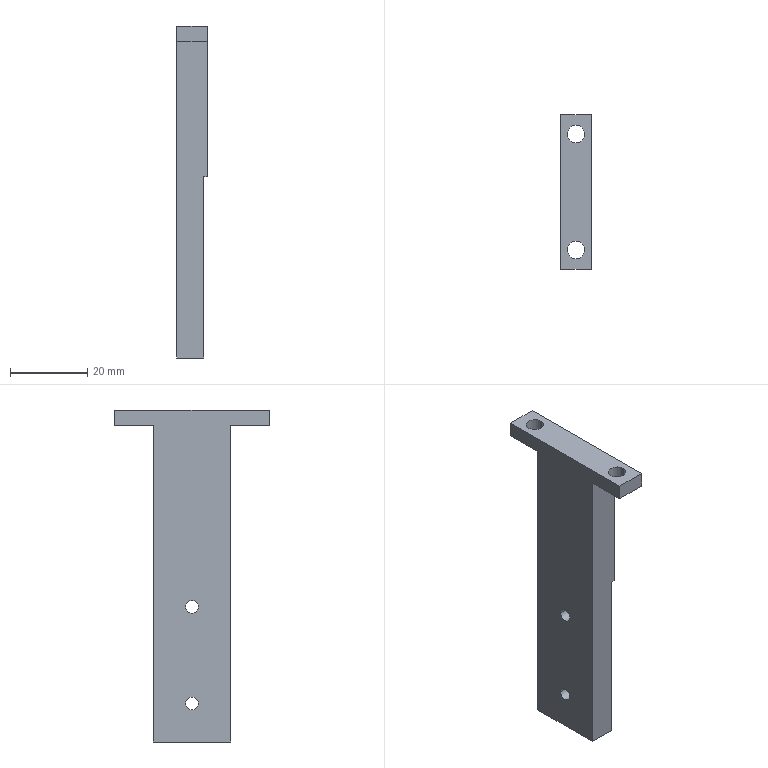Part | NX | 1 solid | 24 faces | box 8 x 40 x 86 mm | volume 13210 mm3 | plane 12 | cylinder 8 | cone 4 | commonest cylinder face diameters 3.3 x4 4.5 x4
STEP:
#1=CARTESIAN_POINT('',(7.,0.,0.));
#2=VERTEX_POINT('',#1);
#3=CARTESIAN_POINT('',(7.,-20.,0.));
#4=VERTEX_POINT('',#3);
#5=CARTESIAN_POINT('',(7.,0.,0.));
#6=DIRECTION('',(0.,-1.,0.));
#7=VECTOR('',#6,1000.);
#8=LINE('',#5,#7);
#9=EDGE_CURVE('',#2,#4,#8,.T.);
#10=ORIENTED_EDGE('',*,*,#9,.T.);
#11=CARTESIAN_POINT('',(0.,-20.,0.));
#12=VERTEX_POINT('',#11);
#13=CARTESIAN_POINT('',(7.,-20.,0.));
#14=DIRECTION('',(-1.,0.,0.));
#15=VECTOR('',#14,1000.);
#16=LINE('',#13,#15);
#17=EDGE_CURVE('',#4,#12,#16,.T.);
#18=ORIENTED_EDGE('',*,*,#17,.T.);
#19=CARTESIAN_POINT('',(0.,0.,0.));
#20=VERTEX_POINT('',#19);
#21=CARTESIAN_POINT('',(0.,0.,0.));
#22=DIRECTION('',(0.,-1.,0.));
#23=VECTOR('',#22,1000.);
#24=LINE('',#21,#23);
#25=EDGE_CURVE('',#20,#12,#24,.T.);
#26=ORIENTED_EDGE('',*,*,#25,.F.);
#27=CARTESIAN_POINT('',(0.,0.,0.));
#28=DIRECTION('',(1.,0.,0.));
#29=VECTOR('',#28,1000.);
#30=LINE('',#27,#29);
#31=EDGE_CURVE('',#20,#2,#30,.T.);
#32=ORIENTED_EDGE('',*,*,#31,.T.);
#33=EDGE_LOOP('',(#10,#18,#26,#32));
#34=FACE_BOUND('',#33,.T.);
#35=CARTESIAN_POINT('',(0.,0.,0.));
#36=DIRECTION('',(0.,0.,1.));
#37=DIRECTION('',(1.,0.,0.));
#38=AXIS2_PLACEMENT_3D('',#35,#36,#37);
#39=PLANE('',#38);
#40=ADVANCED_FACE('',(#34),#39,.F.);
#41=ORIENTED_EDGE('',*,*,#9,.F.);
#42=CARTESIAN_POINT('',(7.,0.,47.));
#43=VERTEX_POINT('',#42);
#44=CARTESIAN_POINT('',(7.,0.,0.));
#45=DIRECTION('',(0.,0.,1.));
#46=VECTOR('',#45,1000.);
#47=LINE('',#44,#46);
#48=EDGE_CURVE('',#2,#43,#47,.T.);
#49=ORIENTED_EDGE('',*,*,#48,.T.);
#50=CARTESIAN_POINT('',(7.,-20.,47.));
#51=VERTEX_POINT('',#50);
#52=CARTESIAN_POINT('',(7.,0.,47.));
#53=DIRECTION('',(0.,-1.,0.));
#54=VECTOR('',#53,1000.);
#55=LINE('',#52,#54);
#56=EDGE_CURVE('',#43,#51,#55,.T.);
#57=ORIENTED_EDGE('',*,*,#56,.T.);
#58=CARTESIAN_POINT('',(7.,-20.,0.));
#59=DIRECTION('',(0.,0.,-1.));
#60=VECTOR('',#59,1000.);
#61=LINE('',#58,#60);
#62=EDGE_CURVE('',#51,#4,#61,.T.);
#63=ORIENTED_EDGE('',*,*,#62,.T.);
#64=EDGE_LOOP('',(#41,#49,#57,#63));
#65=FACE_BOUND('',#64,.T.);
#66=CARTESIAN_POINT('',(7.,-7.685,35.));
#67=VERTEX_POINT('',#66);
#68=CARTESIAN_POINT('',(7.,-12.315,35.));
#69=VERTEX_POINT('',#68);
#70=CARTESIAN_POINT('',(7.,-10.,35.));
#71=DIRECTION('',(1.,0.,0.));
#72=DIRECTION('',(0.,-1.,0.));
#73=AXIS2_PLACEMENT_3D('',#70,#71,#72);
#74=CIRCLE('',#73,2.315);
#75=EDGE_CURVE('',#67,#69,#74,.T.);
#76=ORIENTED_EDGE('',*,*,#75,.F.);
#77=CARTESIAN_POINT('',(7.,-10.,35.));
#78=DIRECTION('',(1.,0.,0.));
#79=DIRECTION('',(0.,-1.,0.));
#80=AXIS2_PLACEMENT_3D('',#77,#78,#79);
#81=CIRCLE('',#80,2.315);
#82=EDGE_CURVE('',#69,#67,#81,.T.);
#83=ORIENTED_EDGE('',*,*,#82,.F.);
#84=EDGE_LOOP('',(#76,#83));
#85=FACE_BOUND('',#84,.T.);
#86=CARTESIAN_POINT('',(7.,-7.685,10.));
#87=VERTEX_POINT('',#86);
#88=CARTESIAN_POINT('',(7.,-12.315,10.));
#89=VERTEX_POINT('',#88);
#90=CARTESIAN_POINT('',(7.,-10.,10.));
#91=DIRECTION('',(1.,0.,0.));
#92=DIRECTION('',(0.,-1.,0.));
#93=AXIS2_PLACEMENT_3D('',#90,#91,#92);
#94=CIRCLE('',#93,2.315);
#95=EDGE_CURVE('',#87,#89,#94,.T.);
#96=ORIENTED_EDGE('',*,*,#95,.F.);
#97=CARTESIAN_POINT('',(7.,-10.,10.));
#98=DIRECTION('',(1.,0.,0.));
#99=DIRECTION('',(0.,-1.,0.));
#100=AXIS2_PLACEMENT_3D('',#97,#98,#99);
#101=CIRCLE('',#100,2.315);
#102=EDGE_CURVE('',#89,#87,#101,.T.);
#103=ORIENTED_EDGE('',*,*,#102,.F.);
#104=EDGE_LOOP('',(#96,#103));
#105=FACE_BOUND('',#104,.T.);
#106=CARTESIAN_POINT('',(7.,0.,0.));
#107=DIRECTION('',(-1.,0.,0.));
#108=DIRECTION('',(0.,0.,1.));
#109=AXIS2_PLACEMENT_3D('',#106,#107,#108);
#110=PLANE('',#109);
#111=ADVANCED_FACE('',(#65,#85,#105),#110,.F.);
#112=CARTESIAN_POINT('',(8.,-20.,82.));
#113=VERTEX_POINT('',#112);
#114=CARTESIAN_POINT('',(0.,-20.,82.));
#115=VERTEX_POINT('',#114);
#116=CARTESIAN_POINT('',(8.,-20.,82.));
#117=DIRECTION('',(-1.,0.,0.));
#118=VECTOR('',#117,1000.);
#119=LINE('',#116,#118);
#120=EDGE_CURVE('',#113,#115,#119,.T.);
#121=ORIENTED_EDGE('',*,*,#120,.T.);
#122=CARTESIAN_POINT('',(0.,-20.,0.));
#123=DIRECTION('',(0.,0.,-1.));
#124=VECTOR('',#123,1000.);
#125=LINE('',#122,#124);
#126=EDGE_CURVE('',#115,#12,#125,.T.);
#127=ORIENTED_EDGE('',*,*,#126,.T.);
#128=ORIENTED_EDGE('',*,*,#17,.F.);
#129=ORIENTED_EDGE('',*,*,#62,.F.);
#130=CARTESIAN_POINT('',(8.,-20.,47.));
#131=VERTEX_POINT('',#130);
#132=CARTESIAN_POINT('',(7.,-20.,47.));
#133=DIRECTION('',(1.,0.,0.));
#134=VECTOR('',#133,1000.);
#135=LINE('',#132,#134);
#136=EDGE_CURVE('',#51,#131,#135,.T.);
#137=ORIENTED_EDGE('',*,*,#136,.T.);
#138=CARTESIAN_POINT('',(8.,-20.,82.));
#139=DIRECTION('',(0.,0.,-1.));
#140=VECTOR('',#139,1000.);
#141=LINE('',#138,#140);
#142=EDGE_CURVE('',#113,#131,#141,.T.);
#143=ORIENTED_EDGE('',*,*,#142,.F.);
#144=EDGE_LOOP('',(#121,#127,#128,#129,#137,#143));
#145=FACE_BOUND('',#144,.T.);
#146=CARTESIAN_POINT('',(0.,-20.,0.));
#147=DIRECTION('',(0.,-1.,0.));
#148=DIRECTION('',(0.,0.,-1.));
#149=AXIS2_PLACEMENT_3D('',#146,#147,#148);
#150=PLANE('',#149);
#151=ADVANCED_FACE('',(#145),#150,.T.);
#152=CARTESIAN_POINT('',(0.,0.,82.));
#153=VERTEX_POINT('',#152);
#154=CARTESIAN_POINT('',(8.,0.,82.));
#155=VERTEX_POINT('',#154);
#156=CARTESIAN_POINT('',(0.,0.,82.));
#157=DIRECTION('',(1.,0.,0.));
#158=VECTOR('',#157,1000.);
#159=LINE('',#156,#158);
#160=EDGE_CURVE('',#153,#155,#159,.T.);
#161=ORIENTED_EDGE('',*,*,#160,.F.);
#162=CARTESIAN_POINT('',(0.,10.,82.));
#163=VERTEX_POINT('',#162);
#164=CARTESIAN_POINT('',(0.,0.,82.));
#165=DIRECTION('',(0.,1.,0.));
#166=VECTOR('',#165,1000.);
#167=LINE('',#164,#166);
#168=EDGE_CURVE('',#153,#163,#167,.T.);
#169=ORIENTED_EDGE('',*,*,#168,.T.);
#170=CARTESIAN_POINT('',(8.,10.,82.));
#171=VERTEX_POINT('',#170);
#172=CARTESIAN_POINT('',(0.,10.,82.));
#173=DIRECTION('',(1.,0.,0.));
#174=VECTOR('',#173,1000.);
#175=LINE('',#172,#174);
#176=EDGE_CURVE('',#163,#171,#175,.T.);
#177=ORIENTED_EDGE('',*,*,#176,.T.);
#178=CARTESIAN_POINT('',(8.,10.,82.));
#179=DIRECTION('',(0.,-1.,0.));
#180=VECTOR('',#179,1000.);
#181=LINE('',#178,#180);
#182=EDGE_CURVE('',#171,#155,#181,.T.);
#183=ORIENTED_EDGE('',*,*,#182,.T.);
#184=EDGE_LOOP('',(#161,#169,#177,#183));
#185=FACE_BOUND('',#184,.T.);
#186=CARTESIAN_POINT('',(1.75,5.,82.));
#187=VERTEX_POINT('',#186);
#188=CARTESIAN_POINT('',(6.25,5.,82.));
#189=VERTEX_POINT('',#188);
#190=CARTESIAN_POINT('',(4.,5.,82.));
#191=DIRECTION('',(0.,0.,-1.));
#192=DIRECTION('',(1.,0.,0.));
#193=AXIS2_PLACEMENT_3D('',#190,#191,#192);
#194=CIRCLE('',#193,2.25);
#195=EDGE_CURVE('',#187,#189,#194,.T.);
#196=ORIENTED_EDGE('',*,*,#195,.F.);
#197=CARTESIAN_POINT('',(4.,5.,82.));
#198=DIRECTION('',(0.,0.,-1.));
#199=DIRECTION('',(1.,0.,0.));
#200=AXIS2_PLACEMENT_3D('',#197,#198,#199);
#201=CIRCLE('',#200,2.25);
#202=EDGE_CURVE('',#189,#187,#201,.T.);
#203=ORIENTED_EDGE('',*,*,#202,.F.);
#204=EDGE_LOOP('',(#196,#203));
#205=FACE_BOUND('',#204,.T.);
#206=CARTESIAN_POINT('',(8.,0.,82.));
#207=DIRECTION('',(0.,0.,-1.));
#208=DIRECTION('',(0.,-1.,0.));
#209=AXIS2_PLACEMENT_3D('',#206,#207,#208);
#210=PLANE('',#209);
#211=ADVANCED_FACE('',(#185,#205),#210,.T.);
#212=CARTESIAN_POINT('',(0.,10.,86.));
#213=VERTEX_POINT('',#212);
#214=CARTESIAN_POINT('',(0.,-30.,86.));
#215=VERTEX_POINT('',#214);
#216=CARTESIAN_POINT('',(0.,0.,86.));
#217=DIRECTION('',(0.,-1.,0.));
#218=VECTOR('',#217,1000.);
#219=LINE('',#216,#218);
#220=EDGE_CURVE('',#213,#215,#219,.T.);
#221=ORIENTED_EDGE('',*,*,#220,.F.);
#222=CARTESIAN_POINT('',(0.,10.,0.));
#223=DIRECTION('',(0.,0.,1.));
#224=VECTOR('',#223,1000.);
#225=LINE('',#222,#224);
#226=EDGE_CURVE('',#163,#213,#225,.T.);
#227=ORIENTED_EDGE('',*,*,#226,.F.);
#228=ORIENTED_EDGE('',*,*,#168,.F.);
#229=CARTESIAN_POINT('',(0.,0.,0.));
#230=DIRECTION('',(0.,0.,1.));
#231=VECTOR('',#230,1000.);
#232=LINE('',#229,#231);
#233=EDGE_CURVE('',#20,#153,#232,.T.);
#234=ORIENTED_EDGE('',*,*,#233,.F.);
#235=ORIENTED_EDGE('',*,*,#25,.T.);
#236=ORIENTED_EDGE('',*,*,#126,.F.);
#237=CARTESIAN_POINT('',(0.,-30.,82.));
#238=VERTEX_POINT('',#237);
#239=CARTESIAN_POINT('',(0.,0.,82.));
#240=DIRECTION('',(0.,1.,0.));
#241=VECTOR('',#240,1000.);
#242=LINE('',#239,#241);
#243=EDGE_CURVE('',#238,#115,#242,.T.);
#244=ORIENTED_EDGE('',*,*,#243,.F.);
#245=CARTESIAN_POINT('',(0.,-30.,0.));
#246=DIRECTION('',(0.,0.,-1.));
#247=VECTOR('',#246,1000.);
#248=LINE('',#245,#247);
#249=EDGE_CURVE('',#215,#238,#248,.T.);
#250=ORIENTED_EDGE('',*,*,#249,.F.);
#251=EDGE_LOOP('',(#221,#227,#228,#234,#235,#236,#244,#250));
#252=FACE_BOUND('',#251,.T.);
#253=CARTESIAN_POINT('',(0.,-11.65,35.));
#254=VERTEX_POINT('',#253);
#255=CARTESIAN_POINT('',(0.,-8.35,35.));
#256=VERTEX_POINT('',#255);
#257=CARTESIAN_POINT('',(0.,-10.,35.));
#258=DIRECTION('',(1.,0.,0.));
#259=DIRECTION('',(0.,-1.,0.));
#260=AXIS2_PLACEMENT_3D('',#257,#258,#259);
#261=CIRCLE('',#260,1.65);
#262=EDGE_CURVE('',#254,#256,#261,.T.);
#263=ORIENTED_EDGE('',*,*,#262,.T.);
#264=CARTESIAN_POINT('',(0.,-10.,35.));
#265=DIRECTION('',(1.,0.,0.));
#266=DIRECTION('',(0.,-1.,0.));
#267=AXIS2_PLACEMENT_3D('',#264,#265,#266);
#268=CIRCLE('',#267,1.65);
#269=EDGE_CURVE('',#256,#254,#268,.T.);
#270=ORIENTED_EDGE('',*,*,#269,.T.);
#271=EDGE_LOOP('',(#263,#270));
#272=FACE_BOUND('',#271,.T.);
#273=CARTESIAN_POINT('',(0.,-11.65,10.));
#274=VERTEX_POINT('',#273);
#275=CARTESIAN_POINT('',(0.,-8.35,10.));
#276=VERTEX_POINT('',#275);
#277=CARTESIAN_POINT('',(0.,-10.,10.));
#278=DIRECTION('',(1.,0.,0.));
#279=DIRECTION('',(0.,-1.,0.));
#280=AXIS2_PLACEMENT_3D('',#277,#278,#279);
#281=CIRCLE('',#280,1.65);
#282=EDGE_CURVE('',#274,#276,#281,.T.);
#283=ORIENTED_EDGE('',*,*,#282,.T.);
#284=CARTESIAN_POINT('',(0.,-10.,10.));
#285=DIRECTION('',(1.,0.,0.));
#286=DIRECTION('',(0.,-1.,0.));
#287=AXIS2_PLACEMENT_3D('',#284,#285,#286);
#288=CIRCLE('',#287,1.65);
#289=EDGE_CURVE('',#276,#274,#288,.T.);
#290=ORIENTED_EDGE('',*,*,#289,.T.);
#291=EDGE_LOOP('',(#283,#290));
#292=FACE_BOUND('',#291,.T.);
#293=CARTESIAN_POINT('',(0.,0.,0.));
#294=DIRECTION('',(-1.,0.,0.));
#295=DIRECTION('',(0.,0.,1.));
#296=AXIS2_PLACEMENT_3D('',#293,#294,#295);
#297=PLANE('',#296);
#298=ADVANCED_FACE('',(#252,#272,#292),#297,.T.);
#299=ORIENTED_EDGE('',*,*,#120,.F.);
#300=CARTESIAN_POINT('',(8.,-30.,82.));
#301=VERTEX_POINT('',#300);
#302=CARTESIAN_POINT('',(8.,-20.,82.));
#303=DIRECTION('',(0.,-1.,0.));
#304=VECTOR('',#303,1000.);
#305=LINE('',#302,#304);
#306=EDGE_CURVE('',#113,#301,#305,.T.);
#307=ORIENTED_EDGE('',*,*,#306,.T.);
#308=CARTESIAN_POINT('',(0.,-30.,82.));
#309=DIRECTION('',(1.,0.,0.));
#310=VECTOR('',#309,1000.);
#311=LINE('',#308,#310);
#312=EDGE_CURVE('',#238,#301,#311,.T.);
#313=ORIENTED_EDGE('',*,*,#312,.F.);
#314=ORIENTED_EDGE('',*,*,#243,.T.);
#315=EDGE_LOOP('',(#299,#307,#313,#314));
#316=FACE_BOUND('',#315,.T.);
#317=CARTESIAN_POINT('',(1.75,-25.,82.));
#318=VERTEX_POINT('',#317);
#319=CARTESIAN_POINT('',(6.25,-25.,82.));
#320=VERTEX_POINT('',#319);
#321=CARTESIAN_POINT('',(4.,-25.,82.));
#322=DIRECTION('',(0.,0.,-1.));
#323=DIRECTION('',(1.,0.,0.));
#324=AXIS2_PLACEMENT_3D('',#321,#322,#323);
#325=CIRCLE('',#324,2.25);
#326=EDGE_CURVE('',#318,#320,#325,.T.);
#327=ORIENTED_EDGE('',*,*,#326,.F.);
#328=CARTESIAN_POINT('',(4.,-25.,82.));
#329=DIRECTION('',(0.,0.,-1.));
#330=DIRECTION('',(1.,0.,0.));
#331=AXIS2_PLACEMENT_3D('',#328,#329,#330);
#332=CIRCLE('',#331,2.25);
#333=EDGE_CURVE('',#320,#318,#332,.T.);
#334=ORIENTED_EDGE('',*,*,#333,.F.);
#335=EDGE_LOOP('',(#327,#334));
#336=FACE_BOUND('',#335,.T.);
#337=CARTESIAN_POINT('',(8.,-30.,82.));
#338=DIRECTION('',(0.,0.,-1.));
#339=DIRECTION('',(0.,-1.,0.));
#340=AXIS2_PLACEMENT_3D('',#337,#338,#339);
#341=PLANE('',#340);
#342=ADVANCED_FACE('',(#316,#336),#341,.T.);
#343=CARTESIAN_POINT('',(8.,-30.,86.));
#344=VERTEX_POINT('',#343);
#345=CARTESIAN_POINT('',(8.,10.,86.));
#346=VERTEX_POINT('',#345);
#347=CARTESIAN_POINT('',(8.,-30.,86.));
#348=DIRECTION('',(0.,1.,0.));
#349=VECTOR('',#348,1000.);
#350=LINE('',#347,#349);
#351=EDGE_CURVE('',#344,#346,#350,.T.);
#352=ORIENTED_EDGE('',*,*,#351,.F.);
#353=CARTESIAN_POINT('',(8.,-30.,82.));
#354=DIRECTION('',(0.,0.,1.));
#355=VECTOR('',#354,1000.);
#356=LINE('',#353,#355);
#357=EDGE_CURVE('',#301,#344,#356,.T.);
#358=ORIENTED_EDGE('',*,*,#357,.F.);
#359=ORIENTED_EDGE('',*,*,#306,.F.);
#360=ORIENTED_EDGE('',*,*,#142,.T.);
#361=CARTESIAN_POINT('',(8.,0.,47.));
#362=VERTEX_POINT('',#361);
#363=CARTESIAN_POINT('',(8.,0.,47.));
#364=DIRECTION('',(0.,-1.,0.));
#365=VECTOR('',#364,1000.);
#366=LINE('',#363,#365);
#367=EDGE_CURVE('',#362,#131,#366,.T.);
#368=ORIENTED_EDGE('',*,*,#367,.F.);
#369=CARTESIAN_POINT('',(8.,0.,82.));
#370=DIRECTION('',(0.,0.,-1.));
#371=VECTOR('',#370,1000.);
#372=LINE('',#369,#371);
#373=EDGE_CURVE('',#155,#362,#372,.T.);
#374=ORIENTED_EDGE('',*,*,#373,.F.);
#375=ORIENTED_EDGE('',*,*,#182,.F.);
#376=CARTESIAN_POINT('',(8.,10.,86.));
#377=DIRECTION('',(0.,0.,-1.));
#378=VECTOR('',#377,1000.);
#379=LINE('',#376,#378);
#380=EDGE_CURVE('',#346,#171,#379,.T.);
#381=ORIENTED_EDGE('',*,*,#380,.F.);
#382=EDGE_LOOP('',(#352,#358,#359,#360,#368,#374,#375,#381));
#383=FACE_BOUND('',#382,.T.);
#384=CARTESIAN_POINT('',(8.,-20.,0.));
#385=DIRECTION('',(1.,0.,0.));
#386=DIRECTION('',(0.,1.,0.));
#387=AXIS2_PLACEMENT_3D('',#384,#385,#386);
#388=PLANE('',#387);
#389=ADVANCED_FACE('',(#383),#388,.T.);
#390=ORIENTED_EDGE('',*,*,#380,.T.);
#391=ORIENTED_EDGE('',*,*,#176,.F.);
#392=ORIENTED_EDGE('',*,*,#226,.T.);
#393=CARTESIAN_POINT('',(0.,10.,86.));
#394=DIRECTION('',(1.,0.,0.));
#395=VECTOR('',#394,1000.);
#396=LINE('',#393,#395);
#397=EDGE_CURVE('',#213,#346,#396,.T.);
#398=ORIENTED_EDGE('',*,*,#397,.T.);
#399=EDGE_LOOP('',(#390,#391,#392,#398));
#400=FACE_BOUND('',#399,.T.);
#401=CARTESIAN_POINT('',(8.,10.,82.));
#402=DIRECTION('',(0.,1.,0.));
#403=DIRECTION('',(1.,0.,0.));
#404=AXIS2_PLACEMENT_3D('',#401,#402,#403);
#405=PLANE('',#404);
#406=ADVANCED_FACE('',(#400),#405,.T.);
#407=ORIENTED_EDGE('',*,*,#351,.T.);
#408=ORIENTED_EDGE('',*,*,#397,.F.);
#409=ORIENTED_EDGE('',*,*,#220,.T.);
#410=CARTESIAN_POINT('',(0.,-30.,86.));
#411=DIRECTION('',(1.,0.,0.));
#412=VECTOR('',#411,1000.);
#413=LINE('',#410,#412);
#414=EDGE_CURVE('',#215,#344,#413,.T.);
#415=ORIENTED_EDGE('',*,*,#414,.T.);
#416=EDGE_LOOP('',(#407,#408,#409,#415));
#417=FACE_BOUND('',#416,.T.);
#418=CARTESIAN_POINT('',(1.75,5.,86.));
#419=VERTEX_POINT('',#418);
#420=CARTESIAN_POINT('',(6.25,5.,86.));
#421=VERTEX_POINT('',#420);
#422=CARTESIAN_POINT('',(4.,5.,86.));
#423=DIRECTION('',(0.,0.,1.));
#424=DIRECTION('',(-1.,0.,0.));
#425=AXIS2_PLACEMENT_3D('',#422,#423,#424);
#426=CIRCLE('',#425,2.25);
#427=EDGE_CURVE('',#419,#421,#426,.T.);
#428=ORIENTED_EDGE('',*,*,#427,.F.);
#429=CARTESIAN_POINT('',(4.,5.,86.));
#430=DIRECTION('',(0.,0.,1.));
#431=DIRECTION('',(-1.,0.,0.));
#432=AXIS2_PLACEMENT_3D('',#429,#430,#431);
#433=CIRCLE('',#432,2.25);
#434=EDGE_CURVE('',#421,#419,#433,.T.);
#435=ORIENTED_EDGE('',*,*,#434,.F.);
#436=EDGE_LOOP('',(#428,#435));
#437=FACE_BOUND('',#436,.T.);
#438=CARTESIAN_POINT('',(6.25,-25.,86.));
#439=VERTEX_POINT('',#438);
#440=CARTESIAN_POINT('',(1.75,-25.,86.));
#441=VERTEX_POINT('',#440);
#442=CARTESIAN_POINT('',(4.,-25.,86.));
#443=DIRECTION('',(0.,0.,1.));
#444=DIRECTION('',(-1.,0.,0.));
#445=AXIS2_PLACEMENT_3D('',#442,#443,#444);
#446=CIRCLE('',#445,2.25);
#447=EDGE_CURVE('',#439,#441,#446,.T.);
#448=ORIENTED_EDGE('',*,*,#447,.F.);
#449=CARTESIAN_POINT('',(4.,-25.,86.));
#450=DIRECTION('',(0.,0.,1.));
#451=DIRECTION('',(-1.,0.,0.));
#452=AXIS2_PLACEMENT_3D('',#449,#450,#451);
#453=CIRCLE('',#452,2.25);
#454=EDGE_CURVE('',#441,#439,#453,.T.);
#455=ORIENTED_EDGE('',*,*,#454,.F.);
#456=EDGE_LOOP('',(#448,#455));
#457=FACE_BOUND('',#456,.T.);
#458=CARTESIAN_POINT('',(0.,0.,86.));
#459=DIRECTION('',(0.,0.,1.));
#460=DIRECTION('',(1.,0.,0.));
#461=AXIS2_PLACEMENT_3D('',#458,#459,#460);
#462=PLANE('',#461);
#463=ADVANCED_FACE('',(#417,#437,#457),#462,.T.);
#464=ORIENTED_EDGE('',*,*,#160,.T.);
#465=ORIENTED_EDGE('',*,*,#373,.T.);
#466=CARTESIAN_POINT('',(7.,0.,47.));
#467=DIRECTION('',(1.,0.,0.));
#468=VECTOR('',#467,1000.);
#469=LINE('',#466,#468);
#470=EDGE_CURVE('',#43,#362,#469,.T.);
#471=ORIENTED_EDGE('',*,*,#470,.F.);
#472=ORIENTED_EDGE('',*,*,#48,.F.);
#473=ORIENTED_EDGE('',*,*,#31,.F.);
#474=ORIENTED_EDGE('',*,*,#233,.T.);
#475=EDGE_LOOP('',(#464,#465,#471,#472,#473,#474));
#476=FACE_BOUND('',#475,.T.);
#477=CARTESIAN_POINT('',(8.,0.,0.));
#478=DIRECTION('',(0.,1.,0.));
#479=DIRECTION('',(1.,0.,0.));
#480=AXIS2_PLACEMENT_3D('',#477,#478,#479);
#481=PLANE('',#480);
#482=ADVANCED_FACE('',(#476),#481,.T.);
#483=ORIENTED_EDGE('',*,*,#136,.F.);
#484=ORIENTED_EDGE('',*,*,#56,.F.);
#485=ORIENTED_EDGE('',*,*,#470,.T.);
#486=ORIENTED_EDGE('',*,*,#367,.T.);
#487=EDGE_LOOP('',(#483,#484,#485,#486));
#488=FACE_BOUND('',#487,.T.);
#489=CARTESIAN_POINT('',(7.,0.,47.));
#490=DIRECTION('',(0.,0.,1.));
#491=DIRECTION('',(1.,0.,0.));
#492=AXIS2_PLACEMENT_3D('',#489,#490,#491);
#493=PLANE('',#492);
#494=ADVANCED_FACE('',(#488),#493,.F.);
#495=ORIENTED_EDGE('',*,*,#427,.T.);
#496=CARTESIAN_POINT('',(6.25,5.,82.));
#497=DIRECTION('',(0.,0.,1.));
#498=VECTOR('',#497,1000.);
#499=LINE('',#496,#498);
#500=EDGE_CURVE('',#189,#421,#499,.T.);
#501=ORIENTED_EDGE('',*,*,#500,.F.);
#502=ORIENTED_EDGE('',*,*,#202,.T.);
#503=CARTESIAN_POINT('',(1.75,5.,82.));
#504=DIRECTION('',(0.,0.,1.));
#505=VECTOR('',#504,1000.);
#506=LINE('',#503,#505);
#507=EDGE_CURVE('',#187,#419,#506,.T.);
#508=ORIENTED_EDGE('',*,*,#507,.T.);
#509=EDGE_LOOP('',(#495,#501,#502,#508));
#510=FACE_BOUND('',#509,.T.);
#511=CARTESIAN_POINT('',(4.,5.,82.));
#512=DIRECTION('',(0.,0.,1.));
#513=DIRECTION('',(1.,0.,0.));
#514=AXIS2_PLACEMENT_3D('',#511,#512,#513);
#515=CYLINDRICAL_SURFACE('',#514,2.25);
#516=ADVANCED_FACE('',(#510),#515,.F.);
#517=ORIENTED_EDGE('',*,*,#447,.T.);
#518=CARTESIAN_POINT('',(1.75,-25.,82.));
#519=DIRECTION('',(0.,0.,1.));
#520=VECTOR('',#519,1000.);
#521=LINE('',#518,#520);
#522=EDGE_CURVE('',#318,#441,#521,.T.);
#523=ORIENTED_EDGE('',*,*,#522,.F.);
#524=ORIENTED_EDGE('',*,*,#326,.T.);
#525=CARTESIAN_POINT('',(6.25,-25.,82.));
#526=DIRECTION('',(0.,0.,1.));
#527=VECTOR('',#526,1000.);
#528=LINE('',#525,#527);
#529=EDGE_CURVE('',#320,#439,#528,.T.);
#530=ORIENTED_EDGE('',*,*,#529,.T.);
#531=EDGE_LOOP('',(#517,#523,#524,#530));
#532=FACE_BOUND('',#531,.T.);
#533=CARTESIAN_POINT('',(4.,-25.,82.));
#534=DIRECTION('',(0.,0.,1.));
#535=DIRECTION('',(1.,0.,0.));
#536=AXIS2_PLACEMENT_3D('',#533,#534,#535);
#537=CYLINDRICAL_SURFACE('',#536,2.25);
#538=ADVANCED_FACE('',(#532),#537,.F.);
#539=ORIENTED_EDGE('',*,*,#357,.T.);
#540=ORIENTED_EDGE('',*,*,#414,.F.);
#541=ORIENTED_EDGE('',*,*,#249,.T.);
#542=ORIENTED_EDGE('',*,*,#312,.T.);
#543=EDGE_LOOP('',(#539,#540,#541,#542));
#544=FACE_BOUND('',#543,.T.);
#545=CARTESIAN_POINT('',(8.,-30.,86.));
#546=DIRECTION('',(0.,-1.,0.));
#547=DIRECTION('',(0.,0.,-1.));
#548=AXIS2_PLACEMENT_3D('',#545,#546,#547);
#549=PLANE('',#548);
#550=ADVANCED_FACE('',(#544),#549,.T.);
#551=ORIENTED_EDGE('',*,*,#262,.F.);
#552=CARTESIAN_POINT('',(6.616,-11.65,35.));
#553=VERTEX_POINT('',#552);
#554=CARTESIAN_POINT('',(7.,-11.65,35.));
#555=DIRECTION('',(1.,0.,0.));
#556=VECTOR('',#555,1000.);
#557=LINE('',#554,#556);
#558=EDGE_CURVE('',#553,#254,#557,.F.);
#559=ORIENTED_EDGE('',*,*,#558,.F.);
#560=CARTESIAN_POINT('',(6.616,-8.35,35.));
#561=VERTEX_POINT('',#560);
#562=CARTESIAN_POINT('',(6.616,-10.,35.));
#563=DIRECTION('',(1.,0.,0.));
#564=DIRECTION('',(0.,-1.,0.));
#565=AXIS2_PLACEMENT_3D('',#562,#563,#564);
#566=CIRCLE('',#565,1.65);
#567=EDGE_CURVE('',#553,#561,#566,.T.);
#568=ORIENTED_EDGE('',*,*,#567,.T.);
#569=CARTESIAN_POINT('',(7.,-8.35,35.));
#570=DIRECTION('',(1.,0.,0.));
#571=VECTOR('',#570,1000.);
#572=LINE('',#569,#571);
#573=EDGE_CURVE('',#561,#256,#572,.F.);
#574=ORIENTED_EDGE('',*,*,#573,.T.);
#575=EDGE_LOOP('',(#551,#559,#568,#574));
#576=FACE_BOUND('',#575,.T.);
#577=CARTESIAN_POINT('',(7.,-10.,35.));
#578=DIRECTION('',(1.,0.,0.));
#579=DIRECTION('',(0.,-1.,0.));
#580=AXIS2_PLACEMENT_3D('',#577,#578,#579);
#581=CYLINDRICAL_SURFACE('',#580,1.65);
#582=ADVANCED_FACE('',(#576),#581,.F.);
#583=ORIENTED_EDGE('',*,*,#75,.T.);
#584=CARTESIAN_POINT('',(6.616,-11.65,35.));
#585=DIRECTION('',(0.5,-0.866,0.));
#586=VECTOR('',#585,1000.);
#587=LINE('',#584,#586);
#588=EDGE_CURVE('',#69,#553,#587,.F.);
#589=ORIENTED_EDGE('',*,*,#588,.T.);
#590=CARTESIAN_POINT('',(6.616,-10.,35.));
#591=DIRECTION('',(1.,0.,0.));
#592=DIRECTION('',(0.,-1.,0.));
#593=AXIS2_PLACEMENT_3D('',#590,#591,#592);
#594=CIRCLE('',#593,1.65);
#595=EDGE_CURVE('',#561,#553,#594,.T.);
#596=ORIENTED_EDGE('',*,*,#595,.F.);
#597=CARTESIAN_POINT('',(6.616,-8.35,35.));
#598=DIRECTION('',(0.5,0.866,0.));
#599=VECTOR('',#598,1000.);
#600=LINE('',#597,#599);
#601=EDGE_CURVE('',#67,#561,#600,.F.);
#602=ORIENTED_EDGE('',*,*,#601,.F.);
#603=EDGE_LOOP('',(#583,#589,#596,#602));
#604=FACE_BOUND('',#603,.T.);
#605=CARTESIAN_POINT('',(6.616,-10.,35.));
#606=DIRECTION('',(1.,0.,0.));
#607=DIRECTION('',(0.,-1.,0.));
#608=AXIS2_PLACEMENT_3D('',#605,#606,#607);
#609=CONICAL_SURFACE('',#608,1.65,1.047);
#610=ADVANCED_FACE('',(#604),#609,.F.);
#611=ORIENTED_EDGE('',*,*,#282,.F.);
#612=CARTESIAN_POINT('',(6.616,-11.65,10.));
#613=VERTEX_POINT('',#612);
#614=CARTESIAN_POINT('',(7.,-11.65,10.));
#615=DIRECTION('',(1.,0.,0.));
#616=VECTOR('',#615,1000.);
#617=LINE('',#614,#616);
#618=EDGE_CURVE('',#613,#274,#617,.F.);
#619=ORIENTED_EDGE('',*,*,#618,.F.);
#620=CARTESIAN_POINT('',(6.616,-8.35,10.));
#621=VERTEX_POINT('',#620);
#622=CARTESIAN_POINT('',(6.616,-10.,10.));
#623=DIRECTION('',(1.,0.,0.));
#624=DIRECTION('',(0.,-1.,0.));
#625=AXIS2_PLACEMENT_3D('',#622,#623,#624);
#626=CIRCLE('',#625,1.65);
#627=EDGE_CURVE('',#613,#621,#626,.T.);
#628=ORIENTED_EDGE('',*,*,#627,.T.);
#629=CARTESIAN_POINT('',(7.,-8.35,10.));
#630=DIRECTION('',(1.,0.,0.));
#631=VECTOR('',#630,1000.);
#632=LINE('',#629,#631);
#633=EDGE_CURVE('',#621,#276,#632,.F.);
#634=ORIENTED_EDGE('',*,*,#633,.T.);
#635=EDGE_LOOP('',(#611,#619,#628,#634));
#636=FACE_BOUND('',#635,.T.);
#637=CARTESIAN_POINT('',(7.,-10.,10.));
#638=DIRECTION('',(1.,0.,0.));
#639=DIRECTION('',(0.,-1.,0.));
#640=AXIS2_PLACEMENT_3D('',#637,#638,#639);
#641=CYLINDRICAL_SURFACE('',#640,1.65);
#642=ADVANCED_FACE('',(#636),#641,.F.);
#643=ORIENTED_EDGE('',*,*,#95,.T.);
#644=CARTESIAN_POINT('',(6.616,-11.65,10.));
#645=DIRECTION('',(0.5,-0.866,0.));
#646=VECTOR('',#645,1000.);
#647=LINE('',#644,#646);
#648=EDGE_CURVE('',#89,#613,#647,.F.);
#649=ORIENTED_EDGE('',*,*,#648,.T.);
#650=CARTESIAN_POINT('',(6.616,-10.,10.));
#651=DIRECTION('',(1.,0.,0.));
#652=DIRECTION('',(0.,-1.,0.));
#653=AXIS2_PLACEMENT_3D('',#650,#651,#652);
#654=CIRCLE('',#653,1.65);
#655=EDGE_CURVE('',#621,#613,#654,.T.);
#656=ORIENTED_EDGE('',*,*,#655,.F.);
#657=CARTESIAN_POINT('',(6.616,-8.35,10.));
#658=DIRECTION('',(0.5,0.866,0.));
#659=VECTOR('',#658,1000.);
#660=LINE('',#657,#659);
#661=EDGE_CURVE('',#87,#621,#660,.F.);
#662=ORIENTED_EDGE('',*,*,#661,.F.);
#663=EDGE_LOOP('',(#643,#649,#656,#662));
#664=FACE_BOUND('',#663,.T.);
#665=CARTESIAN_POINT('',(6.616,-10.,10.));
#666=DIRECTION('',(1.,0.,0.));
#667=DIRECTION('',(0.,-1.,0.));
#668=AXIS2_PLACEMENT_3D('',#665,#666,#667);
#669=CONICAL_SURFACE('',#668,1.65,1.047);
#670=ADVANCED_FACE('',(#664),#669,.F.);
#671=ORIENTED_EDGE('',*,*,#567,.F.);
#672=ORIENTED_EDGE('',*,*,#588,.F.);
#673=ORIENTED_EDGE('',*,*,#82,.T.);
#674=ORIENTED_EDGE('',*,*,#601,.T.);
#675=EDGE_LOOP('',(#671,#672,#673,#674));
#676=FACE_BOUND('',#675,.T.);
#677=CARTESIAN_POINT('',(6.616,-10.,35.));
#678=DIRECTION('',(1.,0.,0.));
#679=DIRECTION('',(0.,-1.,0.));
#680=AXIS2_PLACEMENT_3D('',#677,#678,#679);
#681=CONICAL_SURFACE('',#680,1.65,1.047);
#682=ADVANCED_FACE('',(#676),#681,.F.);
#683=ORIENTED_EDGE('',*,*,#558,.T.);
#684=ORIENTED_EDGE('',*,*,#269,.F.);
#685=ORIENTED_EDGE('',*,*,#573,.F.);
#686=ORIENTED_EDGE('',*,*,#595,.T.);
#687=EDGE_LOOP('',(#683,#684,#685,#686));
#688=FACE_BOUND('',#687,.T.);
#689=CARTESIAN_POINT('',(7.,-10.,35.));
#690=DIRECTION('',(1.,0.,0.));
#691=DIRECTION('',(0.,-1.,0.));
#692=AXIS2_PLACEMENT_3D('',#689,#690,#691);
#693=CYLINDRICAL_SURFACE('',#692,1.65);
#694=ADVANCED_FACE('',(#688),#693,.F.);
#695=ORIENTED_EDGE('',*,*,#618,.T.);
#696=ORIENTED_EDGE('',*,*,#289,.F.);
#697=ORIENTED_EDGE('',*,*,#633,.F.);
#698=ORIENTED_EDGE('',*,*,#655,.T.);
#699=EDGE_LOOP('',(#695,#696,#697,#698));
#700=FACE_BOUND('',#699,.T.);
#701=CARTESIAN_POINT('',(7.,-10.,10.));
#702=DIRECTION('',(1.,0.,0.));
#703=DIRECTION('',(0.,-1.,0.));
#704=AXIS2_PLACEMENT_3D('',#701,#702,#703);
#705=CYLINDRICAL_SURFACE('',#704,1.65);
#706=ADVANCED_FACE('',(#700),#705,.F.);
#707=ORIENTED_EDGE('',*,*,#529,.F.);
#708=ORIENTED_EDGE('',*,*,#333,.T.);
#709=ORIENTED_EDGE('',*,*,#522,.T.);
#710=ORIENTED_EDGE('',*,*,#454,.T.);
#711=EDGE_LOOP('',(#707,#708,#709,#710));
#712=FACE_BOUND('',#711,.T.);
#713=CARTESIAN_POINT('',(4.,-25.,82.));
#714=DIRECTION('',(0.,0.,1.));
#715=DIRECTION('',(1.,0.,0.));
#716=AXIS2_PLACEMENT_3D('',#713,#714,#715);
#717=CYLINDRICAL_SURFACE('',#716,2.25);
#718=ADVANCED_FACE('',(#712),#717,.F.);
#719=ORIENTED_EDGE('',*,*,#627,.F.);
#720=ORIENTED_EDGE('',*,*,#648,.F.);
#721=ORIENTED_EDGE('',*,*,#102,.T.);
#722=ORIENTED_EDGE('',*,*,#661,.T.);
#723=EDGE_LOOP('',(#719,#720,#721,#722));
#724=FACE_BOUND('',#723,.T.);
#725=CARTESIAN_POINT('',(6.616,-10.,10.));
#726=DIRECTION('',(1.,0.,0.));
#727=DIRECTION('',(0.,-1.,0.));
#728=AXIS2_PLACEMENT_3D('',#725,#726,#727);
#729=CONICAL_SURFACE('',#728,1.65,1.047);
#730=ADVANCED_FACE('',(#724),#729,.F.);
#731=ORIENTED_EDGE('',*,*,#195,.T.);
#732=ORIENTED_EDGE('',*,*,#500,.T.);
#733=ORIENTED_EDGE('',*,*,#434,.T.);
#734=ORIENTED_EDGE('',*,*,#507,.F.);
#735=EDGE_LOOP('',(#731,#732,#733,#734));
#736=FACE_BOUND('',#735,.T.);
#737=CARTESIAN_POINT('',(4.,5.,82.));
#738=DIRECTION('',(0.,0.,1.));
#739=DIRECTION('',(1.,0.,0.));
#740=AXIS2_PLACEMENT_3D('',#737,#738,#739);
#741=CYLINDRICAL_SURFACE('',#740,2.25);
#742=ADVANCED_FACE('',(#736),#741,.F.);
#743=CLOSED_SHELL('',(#40,#111,#151,#211,#298,#342,#389,#406,#463,#482,#494,#516,#538,#550,#582,#610,#642,#670,#682,#694,#706,#718,#730,#742));
#744=MANIFOLD_SOLID_BREP('',#743);
#745=(LENGTH_UNIT()NAMED_UNIT(*)SI_UNIT(.MILLI.,.METRE.));
#746=UNCERTAINTY_MEASURE_WITH_UNIT(LENGTH_MEASURE(0.00001),#745,'','');
#747=(NAMED_UNIT(*)PLANE_ANGLE_UNIT()SI_UNIT($,.RADIAN.));
#748=(NAMED_UNIT(*)SI_UNIT($,.STERADIAN.)SOLID_ANGLE_UNIT());
#749=(GEOMETRIC_REPRESENTATION_CONTEXT(3)GLOBAL_UNCERTAINTY_ASSIGNED_CONTEXT((#746))GLOBAL_UNIT_ASSIGNED_CONTEXT((#745,#747,#748))REPRESENTATION_CONTEXT('',''));
#750=ADVANCED_BREP_SHAPE_REPRESENTATION('',(#744),#749);